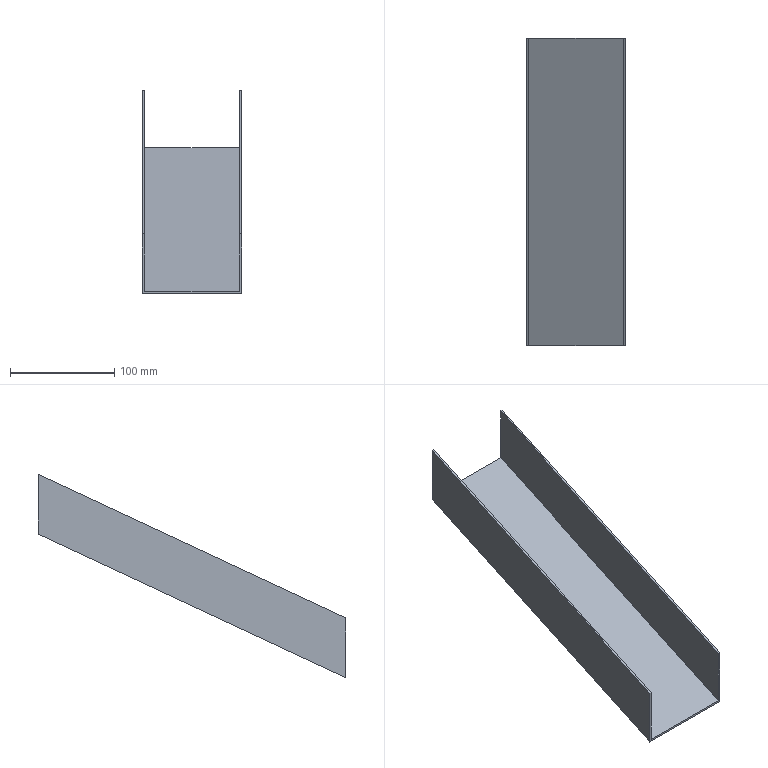Part | NX | features solid 2 | 1 solid | 10 faces | box 95 x 295 x 194.936 mm | volume 126944 mm3 | plane 10
STEP:
#1=CARTESIAN_POINT('',(-132.,-170.,-164.166));
#2=VERTEX_POINT('',#1);
#3=CARTESIAN_POINT('',(-132.,-465.,-301.727));
#4=VERTEX_POINT('',#3);
#5=CARTESIAN_POINT('',(-132.,-283.317,-217.007));
#6=DIRECTION('',(0.,-0.9063,-0.4226));
#7=VECTOR('',#6,1000.);
#8=LINE('',#5,#7);
#9=EDGE_CURVE('',#2,#4,#8,.T.);
#10=ORIENTED_EDGE('',*,*,#9,.F.);
#11=CARTESIAN_POINT('',(-132.,-170.,-219.335));
#12=VERTEX_POINT('',#11);
#13=CARTESIAN_POINT('',(-132.,-170.,-195.));
#14=DIRECTION('',(0.,0.,1.));
#15=VECTOR('',#14,1000.);
#16=LINE('',#13,#15);
#17=EDGE_CURVE('',#12,#2,#16,.T.);
#18=ORIENTED_EDGE('',*,*,#17,.F.);
#19=CARTESIAN_POINT('',(-132.,-465.,-356.896));
#20=VERTEX_POINT('',#19);
#21=CARTESIAN_POINT('',(-132.,-7.673,-143.64));
#22=DIRECTION('',(0.,-0.9063,-0.4226));
#23=VECTOR('',#22,1000.);
#24=LINE('',#21,#23);
#25=EDGE_CURVE('',#12,#20,#24,.T.);
#26=ORIENTED_EDGE('',*,*,#25,.T.);
#27=CARTESIAN_POINT('',(-132.,-465.,-262.322));
#28=DIRECTION('',(0.,0.,1.));
#29=VECTOR('',#28,1000.);
#30=LINE('',#27,#29);
#31=EDGE_CURVE('',#20,#4,#30,.T.);
#32=ORIENTED_EDGE('',*,*,#31,.T.);
#33=EDGE_LOOP('',(#10,#18,#26,#32));
#34=FACE_BOUND('',#33,.T.);
#35=CARTESIAN_POINT('',(-132.,-262.186,-262.322));
#36=DIRECTION('',(-1.,0.,0.));
#37=DIRECTION('',(0.,0.,1.));
#38=AXIS2_PLACEMENT_3D('',#35,#36,#37);
#39=PLANE('',#38);
#40=ADVANCED_FACE('',(#34),#39,.T.);
#41=CARTESIAN_POINT('',(-130.,-170.,-164.166));
#42=VERTEX_POINT('',#41);
#43=CARTESIAN_POINT('',(-130.,-465.,-301.727));
#44=VERTEX_POINT('',#43);
#45=CARTESIAN_POINT('',(-130.,-28.804,-98.325));
#46=DIRECTION('',(0.,-0.9063,-0.4226));
#47=VECTOR('',#46,1000.);
#48=LINE('',#45,#47);
#49=EDGE_CURVE('',#42,#44,#48,.T.);
#50=ORIENTED_EDGE('',*,*,#49,.F.);
#51=CARTESIAN_POINT('',(-225.,-170.,-164.166));
#52=DIRECTION('',(1.,0.,0.));
#53=VECTOR('',#52,1000.);
#54=LINE('',#51,#53);
#55=EDGE_CURVE('',#2,#42,#54,.T.);
#56=ORIENTED_EDGE('',*,*,#55,.F.);
#57=ORIENTED_EDGE('',*,*,#9,.T.);
#58=CARTESIAN_POINT('',(-225.,-465.,-301.727));
#59=DIRECTION('',(-1.,0.,0.));
#60=VECTOR('',#59,1000.);
#61=LINE('',#58,#60);
#62=EDGE_CURVE('',#44,#4,#61,.T.);
#63=ORIENTED_EDGE('',*,*,#62,.F.);
#64=EDGE_LOOP('',(#50,#56,#57,#63));
#65=FACE_BOUND('',#64,.T.);
#66=CARTESIAN_POINT('',(-225.,-28.804,-98.325));
#67=DIRECTION('',(0.,0.4226,-0.9063));
#68=DIRECTION('',(0.,0.9063,0.4226));
#69=AXIS2_PLACEMENT_3D('',#66,#67,#68);
#70=PLANE('',#69);
#71=ADVANCED_FACE('',(#65),#70,.F.);
#72=CARTESIAN_POINT('',(-130.,-170.,-221.542));
#73=VERTEX_POINT('',#72);
#74=CARTESIAN_POINT('',(-130.,-170.,-159.664));
#75=DIRECTION('',(0.,0.,1.));
#76=VECTOR('',#75,1000.);
#77=LINE('',#74,#76);
#78=EDGE_CURVE('',#73,#42,#77,.T.);
#79=ORIENTED_EDGE('',*,*,#78,.T.);
#80=ORIENTED_EDGE('',*,*,#49,.T.);
#81=CARTESIAN_POINT('',(-130.,-465.,-359.102));
#82=VERTEX_POINT('',#81);
#83=CARTESIAN_POINT('',(-130.,-465.,-159.664));
#84=DIRECTION('',(0.,0.,-1.));
#85=VECTOR('',#84,1000.);
#86=LINE('',#83,#85);
#87=EDGE_CURVE('',#44,#82,#86,.T.);
#88=ORIENTED_EDGE('',*,*,#87,.T.);
#89=CARTESIAN_POINT('',(-130.,9.653,-137.768));
#90=DIRECTION('',(0.,0.9063,0.4226));
#91=VECTOR('',#90,1000.);
#92=LINE('',#89,#91);
#93=EDGE_CURVE('',#82,#73,#92,.T.);
#94=ORIENTED_EDGE('',*,*,#93,.T.);
#95=EDGE_LOOP('',(#79,#80,#88,#94));
#96=FACE_BOUND('',#95,.T.);
#97=CARTESIAN_POINT('',(-130.,19.864,-159.664));
#98=DIRECTION('',(1.,0.,0.));
#99=DIRECTION('',(0.,0.342,-0.9397));
#100=AXIS2_PLACEMENT_3D('',#97,#98,#99);
#101=PLANE('',#100);
#102=ADVANCED_FACE('',(#96),#101,.T.);
#103=ORIENTED_EDGE('',*,*,#78,.F.);
#104=CARTESIAN_POINT('',(-225.,-170.,-221.542));
#105=VERTEX_POINT('',#104);
#106=CARTESIAN_POINT('',(-540.,-170.,-221.542));
#107=DIRECTION('',(1.,0.,0.));
#108=VECTOR('',#107,1000.);
#109=LINE('',#106,#108);
#110=EDGE_CURVE('',#105,#73,#109,.T.);
#111=ORIENTED_EDGE('',*,*,#110,.F.);
#112=CARTESIAN_POINT('',(-225.,-170.,-164.166));
#113=VERTEX_POINT('',#112);
#114=CARTESIAN_POINT('',(-225.,-170.,-40.));
#115=DIRECTION('',(0.,0.,1.));
#116=VECTOR('',#115,1000.);
#117=LINE('',#114,#116);
#118=EDGE_CURVE('',#105,#113,#117,.T.);
#119=ORIENTED_EDGE('',*,*,#118,.T.);
#120=CARTESIAN_POINT('',(-223.,-170.,-164.166));
#121=VERTEX_POINT('',#120);
#122=CARTESIAN_POINT('',(-225.,-170.,-164.166));
#123=DIRECTION('',(1.,0.,0.));
#124=VECTOR('',#123,1000.);
#125=LINE('',#122,#124);
#126=EDGE_CURVE('',#113,#121,#125,.T.);
#127=ORIENTED_EDGE('',*,*,#126,.T.);
#128=CARTESIAN_POINT('',(-223.,-170.,-219.335));
#129=VERTEX_POINT('',#128);
#130=CARTESIAN_POINT('',(-223.,-170.,-40.));
#131=DIRECTION('',(0.,0.,1.));
#132=VECTOR('',#131,1000.);
#133=LINE('',#130,#132);
#134=EDGE_CURVE('',#129,#121,#133,.T.);
#135=ORIENTED_EDGE('',*,*,#134,.F.);
#136=CARTESIAN_POINT('',(-140.,-170.,-219.335));
#137=DIRECTION('',(-1.,0.,0.));
#138=VECTOR('',#137,1000.);
#139=LINE('',#136,#138);
#140=EDGE_CURVE('',#12,#129,#139,.T.);
#141=ORIENTED_EDGE('',*,*,#140,.F.);
#142=ORIENTED_EDGE('',*,*,#17,.T.);
#143=ORIENTED_EDGE('',*,*,#55,.T.);
#144=EDGE_LOOP('',(#103,#111,#119,#127,#135,#141,#142,#143));
#145=FACE_BOUND('',#144,.T.);
#146=CARTESIAN_POINT('',(170.,-170.,-195.));
#147=DIRECTION('',(0.,1.,0.));
#148=DIRECTION('',(-1.,0.,0.));
#149=AXIS2_PLACEMENT_3D('',#146,#147,#148);
#150=PLANE('',#149);
#151=ADVANCED_FACE('',(#145),#150,.T.);
#152=CARTESIAN_POINT('',(-225.,-465.,-359.102));
#153=VERTEX_POINT('',#152);
#154=CARTESIAN_POINT('',(-540.,-465.,-359.102));
#155=DIRECTION('',(-1.,0.,0.));
#156=VECTOR('',#155,1000.);
#157=LINE('',#154,#156);
#158=EDGE_CURVE('',#82,#153,#157,.T.);
#159=ORIENTED_EDGE('',*,*,#158,.T.);
#160=CARTESIAN_POINT('',(-225.,-6.828,-145.453));
#161=DIRECTION('',(0.,-0.9063,-0.4226));
#162=VECTOR('',#161,1000.);
#163=LINE('',#160,#162);
#164=EDGE_CURVE('',#105,#153,#163,.T.);
#165=ORIENTED_EDGE('',*,*,#164,.F.);
#166=ORIENTED_EDGE('',*,*,#110,.T.);
#167=ORIENTED_EDGE('',*,*,#93,.F.);
#168=EDGE_LOOP('',(#159,#165,#166,#167));
#169=FACE_BOUND('',#168,.T.);
#170=CARTESIAN_POINT('',(-540.,-6.828,-145.453));
#171=DIRECTION('',(0.,0.4226,-0.9063));
#172=DIRECTION('',(0.,0.9063,0.4226));
#173=AXIS2_PLACEMENT_3D('',#170,#171,#172);
#174=PLANE('',#173);
#175=ADVANCED_FACE('',(#169),#174,.T.);
#176=CARTESIAN_POINT('',(-223.,-465.,-356.896));
#177=VERTEX_POINT('',#176);
#178=CARTESIAN_POINT('',(-910.,-465.,-356.896));
#179=DIRECTION('',(-1.,0.,0.));
#180=VECTOR('',#179,1000.);
#181=LINE('',#178,#180);
#182=EDGE_CURVE('',#20,#177,#181,.T.);
#183=ORIENTED_EDGE('',*,*,#182,.T.);
#184=CARTESIAN_POINT('',(-223.,-465.,-301.727));
#185=VERTEX_POINT('',#184);
#186=CARTESIAN_POINT('',(-223.,-465.,-105.));
#187=DIRECTION('',(0.,0.,1.));
#188=VECTOR('',#187,1000.);
#189=LINE('',#186,#188);
#190=EDGE_CURVE('',#177,#185,#189,.T.);
#191=ORIENTED_EDGE('',*,*,#190,.T.);
#192=CARTESIAN_POINT('',(-225.,-465.,-301.727));
#193=VERTEX_POINT('',#192);
#194=CARTESIAN_POINT('',(-910.,-465.,-301.727));
#195=DIRECTION('',(1.,0.,0.));
#196=VECTOR('',#195,1000.);
#197=LINE('',#194,#196);
#198=EDGE_CURVE('',#193,#185,#197,.T.);
#199=ORIENTED_EDGE('',*,*,#198,.F.);
#200=CARTESIAN_POINT('',(-225.,-465.,-105.));
#201=DIRECTION('',(0.,0.,1.));
#202=VECTOR('',#201,1000.);
#203=LINE('',#200,#202);
#204=EDGE_CURVE('',#153,#193,#203,.T.);
#205=ORIENTED_EDGE('',*,*,#204,.F.);
#206=ORIENTED_EDGE('',*,*,#158,.F.);
#207=ORIENTED_EDGE('',*,*,#87,.F.);
#208=ORIENTED_EDGE('',*,*,#62,.T.);
#209=ORIENTED_EDGE('',*,*,#31,.F.);
#210=EDGE_LOOP('',(#183,#191,#199,#205,#206,#207,#208,#209));
#211=FACE_BOUND('',#210,.T.);
#212=CARTESIAN_POINT('',(-910.,-465.,-105.));
#213=DIRECTION('',(0.,-1.,0.));
#214=DIRECTION('',(0.,0.,-1.));
#215=AXIS2_PLACEMENT_3D('',#212,#213,#214);
#216=PLANE('',#215);
#217=ADVANCED_FACE('',(#211),#216,.T.);
#218=CARTESIAN_POINT('',(-223.,-7.673,-143.64));
#219=DIRECTION('',(0.,0.9063,0.4226));
#220=VECTOR('',#219,1000.);
#221=LINE('',#218,#220);
#222=EDGE_CURVE('',#177,#129,#221,.T.);
#223=ORIENTED_EDGE('',*,*,#222,.F.);
#224=ORIENTED_EDGE('',*,*,#182,.F.);
#225=ORIENTED_EDGE('',*,*,#25,.F.);
#226=ORIENTED_EDGE('',*,*,#140,.T.);
#227=EDGE_LOOP('',(#223,#224,#225,#226));
#228=FACE_BOUND('',#227,.T.);
#229=CARTESIAN_POINT('',(-140.,-7.673,-143.64));
#230=DIRECTION('',(0.,-0.4226,0.9063));
#231=DIRECTION('',(0.,-0.9063,-0.4226));
#232=AXIS2_PLACEMENT_3D('',#229,#230,#231);
#233=PLANE('',#232);
#234=ADVANCED_FACE('',(#228),#233,.T.);
#235=ORIENTED_EDGE('',*,*,#204,.T.);
#236=CARTESIAN_POINT('',(-225.,-56.73,-111.347));
#237=DIRECTION('',(0.,0.9063,0.4226));
#238=VECTOR('',#237,1000.);
#239=LINE('',#236,#238);
#240=EDGE_CURVE('',#193,#113,#239,.T.);
#241=ORIENTED_EDGE('',*,*,#240,.T.);
#242=ORIENTED_EDGE('',*,*,#118,.F.);
#243=ORIENTED_EDGE('',*,*,#164,.T.);
#244=EDGE_LOOP('',(#235,#241,#242,#243));
#245=FACE_BOUND('',#244,.T.);
#246=CARTESIAN_POINT('',(-225.,-90.,-40.));
#247=DIRECTION('',(1.,0.,0.));
#248=DIRECTION('',(0.,0.,-1.));
#249=AXIS2_PLACEMENT_3D('',#246,#247,#248);
#250=PLANE('',#249);
#251=ADVANCED_FACE('',(#245),#250,.F.);
#252=CARTESIAN_POINT('',(-223.,-56.73,-111.347));
#253=DIRECTION('',(0.,0.9063,0.4226));
#254=VECTOR('',#253,1000.);
#255=LINE('',#252,#254);
#256=EDGE_CURVE('',#185,#121,#255,.T.);
#257=ORIENTED_EDGE('',*,*,#256,.T.);
#258=ORIENTED_EDGE('',*,*,#126,.F.);
#259=ORIENTED_EDGE('',*,*,#240,.F.);
#260=ORIENTED_EDGE('',*,*,#198,.T.);
#261=EDGE_LOOP('',(#257,#258,#259,#260));
#262=FACE_BOUND('',#261,.T.);
#263=CARTESIAN_POINT('',(-225.,-28.804,-98.325));
#264=DIRECTION('',(0.,0.4226,-0.9063));
#265=DIRECTION('',(0.,0.9063,0.4226));
#266=AXIS2_PLACEMENT_3D('',#263,#264,#265);
#267=PLANE('',#266);
#268=ADVANCED_FACE('',(#262),#267,.F.);
#269=ORIENTED_EDGE('',*,*,#190,.F.);
#270=ORIENTED_EDGE('',*,*,#222,.T.);
#271=ORIENTED_EDGE('',*,*,#134,.T.);
#272=ORIENTED_EDGE('',*,*,#256,.F.);
#273=EDGE_LOOP('',(#269,#270,#271,#272));
#274=FACE_BOUND('',#273,.T.);
#275=CARTESIAN_POINT('',(-223.,-90.,-40.));
#276=DIRECTION('',(1.,0.,0.));
#277=DIRECTION('',(0.,0.,-1.));
#278=AXIS2_PLACEMENT_3D('',#275,#276,#277);
#279=PLANE('',#278);
#280=ADVANCED_FACE('',(#274),#279,.T.);
#281=CLOSED_SHELL('',(#40,#71,#102,#151,#175,#217,#234,#251,#268,#280));
#282=MANIFOLD_SOLID_BREP('',#281);
#283=(LENGTH_UNIT()NAMED_UNIT(*)SI_UNIT(.MILLI.,.METRE.));
#284=UNCERTAINTY_MEASURE_WITH_UNIT(LENGTH_MEASURE(0.00001),#283,'','');
#285=(NAMED_UNIT(*)PLANE_ANGLE_UNIT()SI_UNIT($,.RADIAN.));
#286=(NAMED_UNIT(*)SI_UNIT($,.STERADIAN.)SOLID_ANGLE_UNIT());
#287=(GEOMETRIC_REPRESENTATION_CONTEXT(3)GLOBAL_UNCERTAINTY_ASSIGNED_CONTEXT((#284))GLOBAL_UNIT_ASSIGNED_CONTEXT((#283,#285,#286))REPRESENTATION_CONTEXT('',''));
#288=ADVANCED_BREP_SHAPE_REPRESENTATION('',(#282),#287);